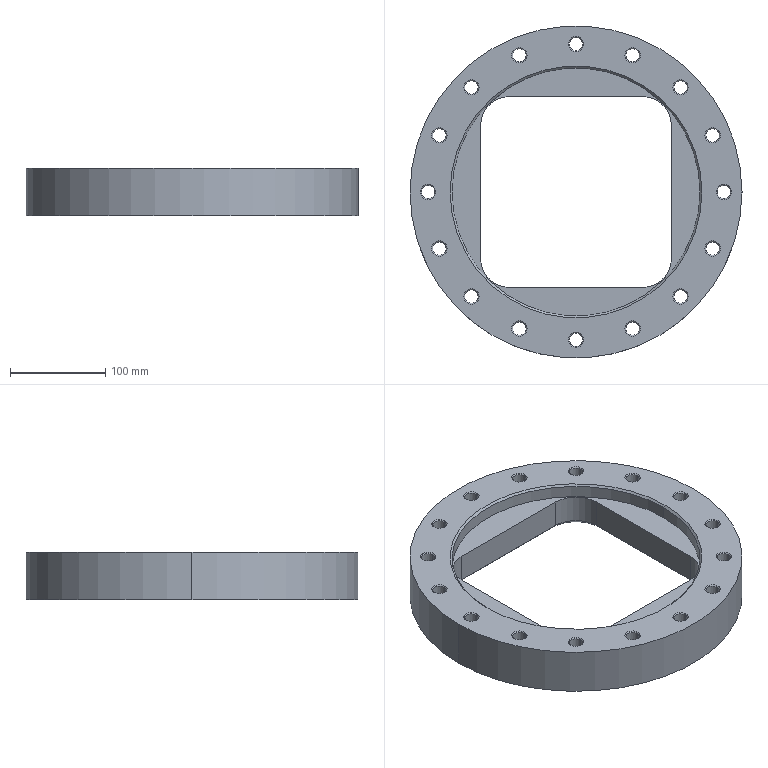Part | SolidWorks | features Chamfer 2, ICE 2, 3DProfileFeature 1, CirPattern 1, Extrusion 1, HoleWzd 1 | 1 solid | 89 faces | box 348 x 348 x 50 mm | volume 2451722 mm3 | cylinder 40 | cone 38 | plane 11 | commonest cylinder face diameters 14 x32 60 x4 260 x2 348 x2